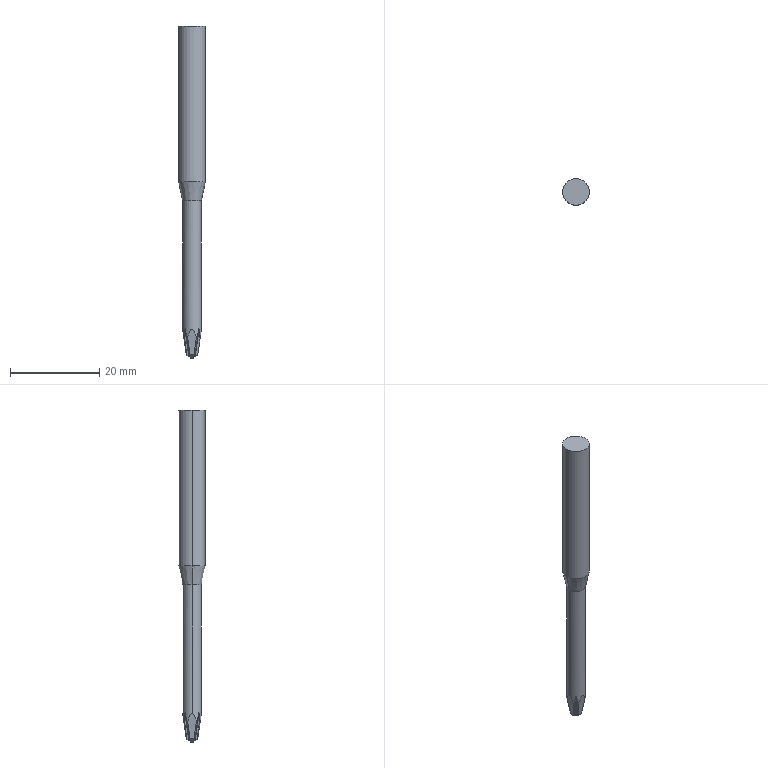Part | SolidWorks | features Revolution 2, Chamfer 1, Fillet 1, ICE 1 | 1 solid | 37 faces | box 6 x 6 x 74.531 mm | volume 1533 mm3 | plane 21 | cone 8 | cylinder 8 | commonest cylinder face diameters 0.4 x4 4.2 x2 6 x2